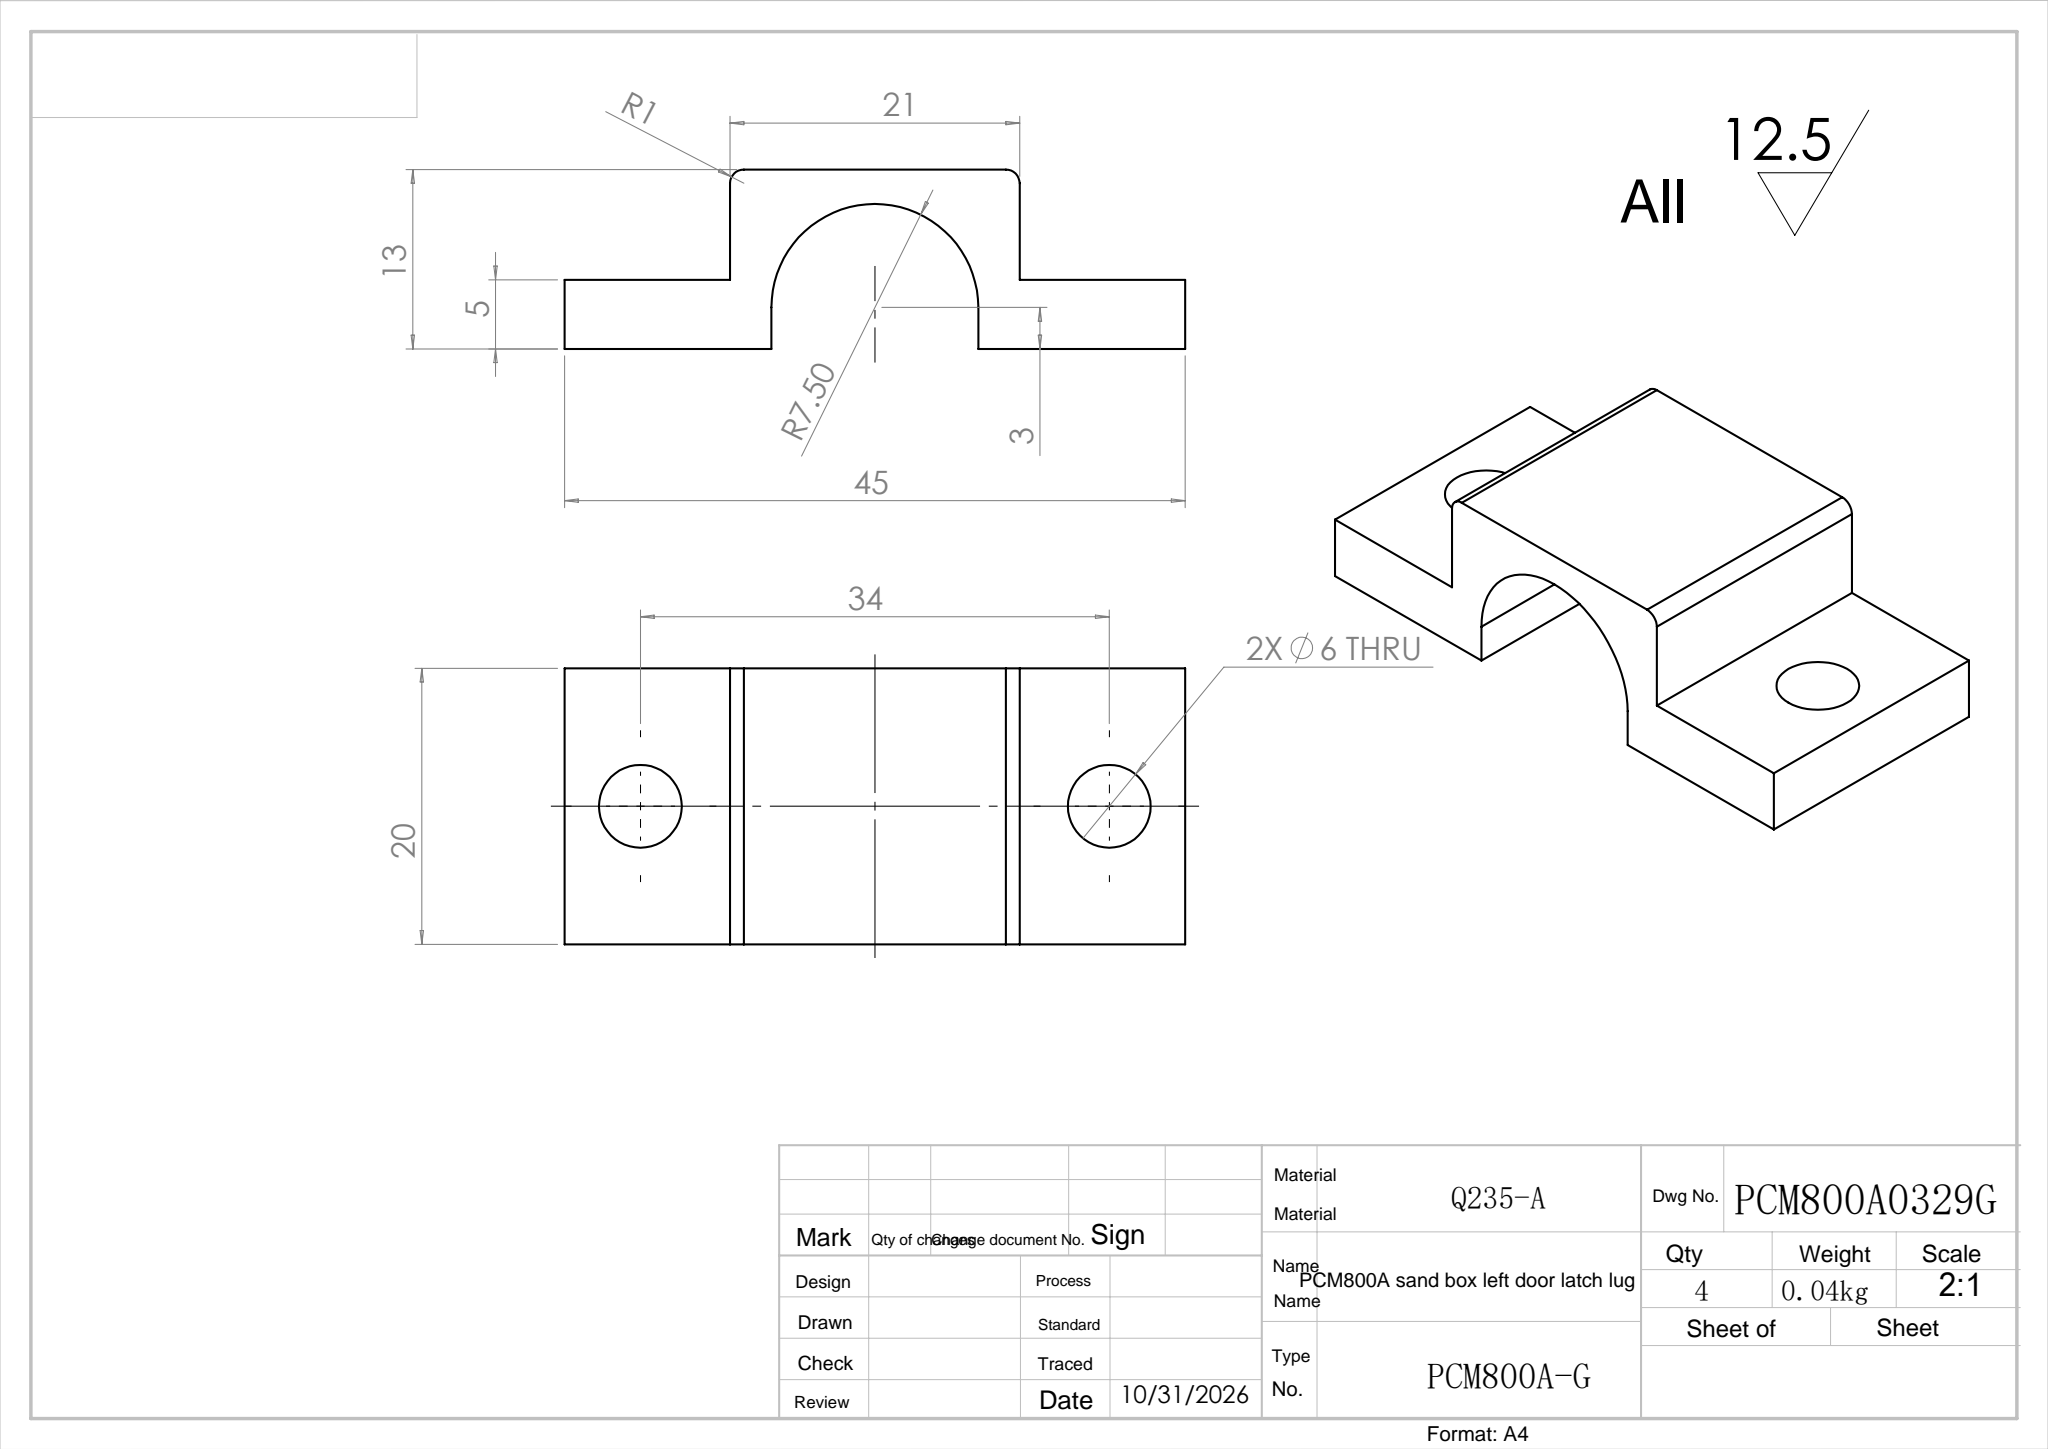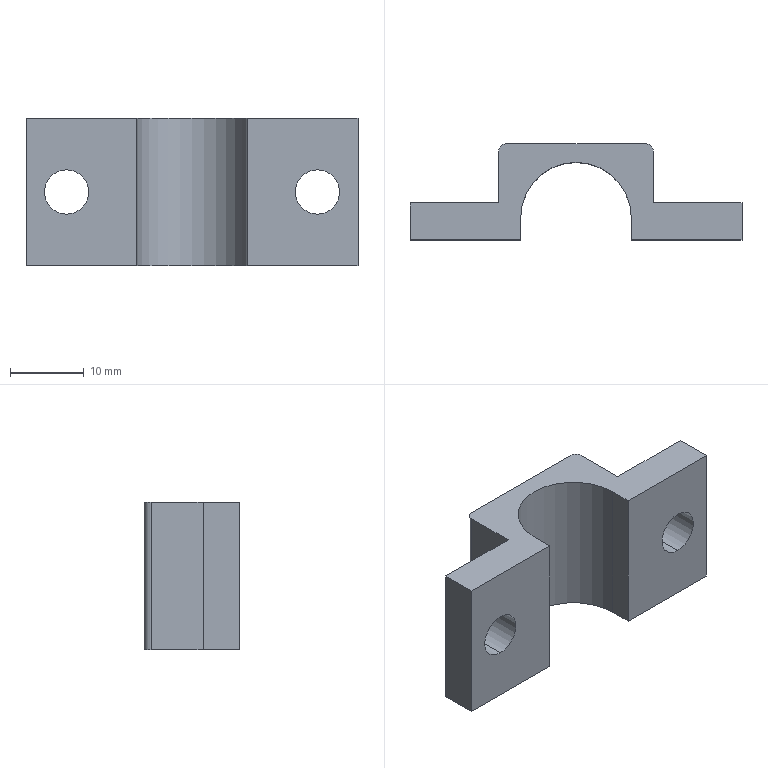Part | SolidWorks | features Extrusion 1, Fillet 1, ICE 1 | 1 solid | 20 faces | box 45 x 13 x 20 mm | volume 4902 mm3 | plane 13 | cylinder 7 | commonest cylinder face diameters 6 x4 2 x2 15 x1
STEP:
#1=CARTESIAN_POINT('',(39.5,-5.,7.));
#2=VERTEX_POINT('',#1);
#3=CARTESIAN_POINT('',(39.5,-5.,13.));
#4=VERTEX_POINT('',#3);
#5=CARTESIAN_POINT('',(39.5,-5.,10.));
#6=DIRECTION('',(0.,1.,0.));
#7=DIRECTION('',(0.,0.,1.));
#8=AXIS2_PLACEMENT_3D('',#5,#6,#7);
#9=CIRCLE('',#8,3.);
#10=EDGE_CURVE('',#2,#4,#9,.T.);
#11=ORIENTED_EDGE('',*,*,#10,.F.);
#12=CARTESIAN_POINT('',(39.5,0.,7.));
#13=VERTEX_POINT('',#12);
#14=CARTESIAN_POINT('',(39.5,-5.,7.));
#15=DIRECTION('',(0.,1.,0.));
#16=VECTOR('',#15,1000.);
#17=LINE('',#14,#16);
#18=EDGE_CURVE('',#2,#13,#17,.T.);
#19=ORIENTED_EDGE('',*,*,#18,.T.);
#20=CARTESIAN_POINT('',(39.5,0.,13.));
#21=VERTEX_POINT('',#20);
#22=CARTESIAN_POINT('',(39.5,0.,10.));
#23=DIRECTION('',(0.,1.,0.));
#24=DIRECTION('',(0.,0.,1.));
#25=AXIS2_PLACEMENT_3D('',#22,#23,#24);
#26=CIRCLE('',#25,3.);
#27=EDGE_CURVE('',#13,#21,#26,.T.);
#28=ORIENTED_EDGE('',*,*,#27,.T.);
#29=CARTESIAN_POINT('',(39.5,-5.,13.));
#30=DIRECTION('',(0.,1.,0.));
#31=VECTOR('',#30,1000.);
#32=LINE('',#29,#31);
#33=EDGE_CURVE('',#4,#21,#32,.T.);
#34=ORIENTED_EDGE('',*,*,#33,.F.);
#35=EDGE_LOOP('',(#11,#19,#28,#34));
#36=FACE_OUTER_BOUND('',#35,.T.);
#37=CARTESIAN_POINT('',(39.5,-5.,10.));
#38=DIRECTION('',(0.,1.,0.));
#39=DIRECTION('',(0.,0.,1.));
#40=AXIS2_PLACEMENT_3D('',#37,#38,#39);
#41=CYLINDRICAL_SURFACE('',#40,3.);
#42=ADVANCED_FACE('',(#36),#41,.F.);
#43=CARTESIAN_POINT('',(5.5,-5.,7.));
#44=VERTEX_POINT('',#43);
#45=CARTESIAN_POINT('',(5.5,-5.,13.));
#46=VERTEX_POINT('',#45);
#47=CARTESIAN_POINT('',(5.5,-5.,10.));
#48=DIRECTION('',(0.,1.,0.));
#49=DIRECTION('',(0.,0.,1.));
#50=AXIS2_PLACEMENT_3D('',#47,#48,#49);
#51=CIRCLE('',#50,3.);
#52=EDGE_CURVE('',#44,#46,#51,.T.);
#53=ORIENTED_EDGE('',*,*,#52,.F.);
#54=CARTESIAN_POINT('',(5.5,0.,7.));
#55=VERTEX_POINT('',#54);
#56=CARTESIAN_POINT('',(5.5,-5.,7.));
#57=DIRECTION('',(0.,1.,0.));
#58=VECTOR('',#57,1000.);
#59=LINE('',#56,#58);
#60=EDGE_CURVE('',#44,#55,#59,.T.);
#61=ORIENTED_EDGE('',*,*,#60,.T.);
#62=CARTESIAN_POINT('',(5.5,0.,13.));
#63=VERTEX_POINT('',#62);
#64=CARTESIAN_POINT('',(5.5,0.,10.));
#65=DIRECTION('',(0.,1.,0.));
#66=DIRECTION('',(0.,0.,1.));
#67=AXIS2_PLACEMENT_3D('',#64,#65,#66);
#68=CIRCLE('',#67,3.);
#69=EDGE_CURVE('',#55,#63,#68,.T.);
#70=ORIENTED_EDGE('',*,*,#69,.T.);
#71=CARTESIAN_POINT('',(5.5,-5.,13.));
#72=DIRECTION('',(0.,1.,0.));
#73=VECTOR('',#72,1000.);
#74=LINE('',#71,#73);
#75=EDGE_CURVE('',#46,#63,#74,.T.);
#76=ORIENTED_EDGE('',*,*,#75,.F.);
#77=EDGE_LOOP('',(#53,#61,#70,#76));
#78=FACE_OUTER_BOUND('',#77,.T.);
#79=CARTESIAN_POINT('',(5.5,-5.,10.));
#80=DIRECTION('',(0.,1.,0.));
#81=DIRECTION('',(0.,0.,1.));
#82=AXIS2_PLACEMENT_3D('',#79,#80,#81);
#83=CYLINDRICAL_SURFACE('',#82,3.);
#84=ADVANCED_FACE('',(#78),#83,.F.);
#85=CARTESIAN_POINT('',(0.,0.,0.));
#86=VERTEX_POINT('',#85);
#87=CARTESIAN_POINT('',(0.,-5.,0.));
#88=VERTEX_POINT('',#87);
#89=CARTESIAN_POINT('',(0.,-5.,0.));
#90=DIRECTION('',(0.,-1.,0.));
#91=VECTOR('',#90,1000.);
#92=LINE('',#89,#91);
#93=EDGE_CURVE('',#86,#88,#92,.T.);
#94=ORIENTED_EDGE('',*,*,#93,.T.);
#95=CARTESIAN_POINT('',(0.,-5.,20.));
#96=VERTEX_POINT('',#95);
#97=CARTESIAN_POINT('',(0.,-5.,20.));
#98=DIRECTION('',(0.,0.,-1.));
#99=VECTOR('',#98,1000.);
#100=LINE('',#97,#99);
#101=EDGE_CURVE('',#96,#88,#100,.T.);
#102=ORIENTED_EDGE('',*,*,#101,.F.);
#103=CARTESIAN_POINT('',(0.,0.,20.));
#104=VERTEX_POINT('',#103);
#105=CARTESIAN_POINT('',(0.,-5.,20.));
#106=DIRECTION('',(0.,-1.,0.));
#107=VECTOR('',#106,1000.);
#108=LINE('',#105,#107);
#109=EDGE_CURVE('',#104,#96,#108,.T.);
#110=ORIENTED_EDGE('',*,*,#109,.F.);
#111=CARTESIAN_POINT('',(0.,0.,20.));
#112=DIRECTION('',(0.,0.,-1.));
#113=VECTOR('',#112,1000.);
#114=LINE('',#111,#113);
#115=EDGE_CURVE('',#104,#86,#114,.T.);
#116=ORIENTED_EDGE('',*,*,#115,.T.);
#117=EDGE_LOOP('',(#94,#102,#110,#116));
#118=FACE_OUTER_BOUND('',#117,.T.);
#119=CARTESIAN_POINT('',(0.,-5.,20.));
#120=DIRECTION('',(1.,0.,0.));
#121=DIRECTION('',(0.,0.,-1.));
#122=AXIS2_PLACEMENT_3D('',#119,#120,#121);
#123=PLANE('',#122);
#124=ADVANCED_FACE('',(#118),#123,.F.);
#125=CARTESIAN_POINT('',(5.5,-5.,10.));
#126=DIRECTION('',(0.,1.,0.));
#127=DIRECTION('',(0.,0.,1.));
#128=AXIS2_PLACEMENT_3D('',#125,#126,#127);
#129=CIRCLE('',#128,3.);
#130=EDGE_CURVE('',#46,#44,#129,.T.);
#131=ORIENTED_EDGE('',*,*,#130,.T.);
#132=ORIENTED_EDGE('',*,*,#52,.T.);
#133=EDGE_LOOP('',(#131,#132));
#134=FACE_BOUND('',#133,.T.);
#135=CARTESIAN_POINT('',(15.,-5.,0.));
#136=VERTEX_POINT('',#135);
#137=CARTESIAN_POINT('',(15.,-5.,0.));
#138=DIRECTION('',(1.,0.,0.));
#139=VECTOR('',#138,1000.);
#140=LINE('',#137,#139);
#141=EDGE_CURVE('',#88,#136,#140,.T.);
#142=ORIENTED_EDGE('',*,*,#141,.T.);
#143=CARTESIAN_POINT('',(15.,-5.,20.));
#144=VERTEX_POINT('',#143);
#145=CARTESIAN_POINT('',(15.,-5.,20.));
#146=DIRECTION('',(0.,0.,-1.));
#147=VECTOR('',#146,1000.);
#148=LINE('',#145,#147);
#149=EDGE_CURVE('',#144,#136,#148,.T.);
#150=ORIENTED_EDGE('',*,*,#149,.F.);
#151=CARTESIAN_POINT('',(15.,-5.,20.));
#152=DIRECTION('',(1.,0.,0.));
#153=VECTOR('',#152,1000.);
#154=LINE('',#151,#153);
#155=EDGE_CURVE('',#96,#144,#154,.T.);
#156=ORIENTED_EDGE('',*,*,#155,.F.);
#157=ORIENTED_EDGE('',*,*,#101,.T.);
#158=EDGE_LOOP('',(#142,#150,#156,#157));
#159=FACE_OUTER_BOUND('',#158,.T.);
#160=CARTESIAN_POINT('',(15.,-5.,20.));
#161=DIRECTION('',(0.,1.,0.));
#162=DIRECTION('',(-1.,0.,0.));
#163=AXIS2_PLACEMENT_3D('',#160,#161,#162);
#164=PLANE('',#163);
#165=ADVANCED_FACE('',(#134,#159),#164,.F.);
#166=CARTESIAN_POINT('',(15.,-2.,0.));
#167=VERTEX_POINT('',#166);
#168=CARTESIAN_POINT('',(15.,-2.,0.));
#169=DIRECTION('',(0.,1.,0.));
#170=VECTOR('',#169,1000.);
#171=LINE('',#168,#170);
#172=EDGE_CURVE('',#136,#167,#171,.T.);
#173=ORIENTED_EDGE('',*,*,#172,.T.);
#174=CARTESIAN_POINT('',(15.,-2.,20.));
#175=VERTEX_POINT('',#174);
#176=CARTESIAN_POINT('',(15.,-2.,20.));
#177=DIRECTION('',(0.,0.,-1.));
#178=VECTOR('',#177,1000.);
#179=LINE('',#176,#178);
#180=EDGE_CURVE('',#175,#167,#179,.T.);
#181=ORIENTED_EDGE('',*,*,#180,.F.);
#182=CARTESIAN_POINT('',(15.,-2.,20.));
#183=DIRECTION('',(0.,1.,0.));
#184=VECTOR('',#183,1000.);
#185=LINE('',#182,#184);
#186=EDGE_CURVE('',#144,#175,#185,.T.);
#187=ORIENTED_EDGE('',*,*,#186,.F.);
#188=ORIENTED_EDGE('',*,*,#149,.T.);
#189=EDGE_LOOP('',(#173,#181,#187,#188));
#190=FACE_OUTER_BOUND('',#189,.T.);
#191=CARTESIAN_POINT('',(15.,-2.,20.));
#192=DIRECTION('',(-1.,0.,0.));
#193=DIRECTION('',(0.,0.,1.));
#194=AXIS2_PLACEMENT_3D('',#191,#192,#193);
#195=PLANE('',#194);
#196=ADVANCED_FACE('',(#190),#195,.F.);
#197=CARTESIAN_POINT('',(30.,-2.,0.));
#198=VERTEX_POINT('',#197);
#199=CARTESIAN_POINT('',(22.5,-2.,0.));
#200=DIRECTION('',(0.,0.,-1.));
#201=DIRECTION('',(1.,0.,0.));
#202=AXIS2_PLACEMENT_3D('',#199,#200,#201);
#203=CIRCLE('',#202,7.5);
#204=EDGE_CURVE('',#167,#198,#203,.T.);
#205=ORIENTED_EDGE('',*,*,#204,.T.);
#206=CARTESIAN_POINT('',(30.,-2.,20.));
#207=VERTEX_POINT('',#206);
#208=CARTESIAN_POINT('',(30.,-2.,20.));
#209=DIRECTION('',(0.,0.,-1.));
#210=VECTOR('',#209,1000.);
#211=LINE('',#208,#210);
#212=EDGE_CURVE('',#207,#198,#211,.T.);
#213=ORIENTED_EDGE('',*,*,#212,.F.);
#214=CARTESIAN_POINT('',(22.5,-2.,20.));
#215=DIRECTION('',(0.,0.,-1.));
#216=DIRECTION('',(1.,0.,0.));
#217=AXIS2_PLACEMENT_3D('',#214,#215,#216);
#218=CIRCLE('',#217,7.5);
#219=EDGE_CURVE('',#175,#207,#218,.T.);
#220=ORIENTED_EDGE('',*,*,#219,.F.);
#221=ORIENTED_EDGE('',*,*,#180,.T.);
#222=EDGE_LOOP('',(#205,#213,#220,#221));
#223=FACE_OUTER_BOUND('',#222,.T.);
#224=CARTESIAN_POINT('',(22.5,-2.,20.));
#225=DIRECTION('',(0.,0.,-1.));
#226=DIRECTION('',(-1.,0.,0.));
#227=AXIS2_PLACEMENT_3D('',#224,#225,#226);
#228=CYLINDRICAL_SURFACE('',#227,7.5);
#229=ADVANCED_FACE('',(#223),#228,.F.);
#230=CARTESIAN_POINT('',(30.,-5.,0.));
#231=VERTEX_POINT('',#230);
#232=CARTESIAN_POINT('',(30.,-2.,0.));
#233=DIRECTION('',(0.,-1.,0.));
#234=VECTOR('',#233,1000.);
#235=LINE('',#232,#234);
#236=EDGE_CURVE('',#198,#231,#235,.T.);
#237=ORIENTED_EDGE('',*,*,#236,.T.);
#238=CARTESIAN_POINT('',(30.,-5.,20.));
#239=VERTEX_POINT('',#238);
#240=CARTESIAN_POINT('',(30.,-5.,20.));
#241=DIRECTION('',(0.,0.,-1.));
#242=VECTOR('',#241,1000.);
#243=LINE('',#240,#242);
#244=EDGE_CURVE('',#239,#231,#243,.T.);
#245=ORIENTED_EDGE('',*,*,#244,.F.);
#246=CARTESIAN_POINT('',(30.,-2.,20.));
#247=DIRECTION('',(0.,-1.,0.));
#248=VECTOR('',#247,1000.);
#249=LINE('',#246,#248);
#250=EDGE_CURVE('',#207,#239,#249,.T.);
#251=ORIENTED_EDGE('',*,*,#250,.F.);
#252=ORIENTED_EDGE('',*,*,#212,.T.);
#253=EDGE_LOOP('',(#237,#245,#251,#252));
#254=FACE_OUTER_BOUND('',#253,.T.);
#255=CARTESIAN_POINT('',(30.,-2.,20.));
#256=DIRECTION('',(1.,0.,0.));
#257=DIRECTION('',(0.,0.,-1.));
#258=AXIS2_PLACEMENT_3D('',#255,#256,#257);
#259=PLANE('',#258);
#260=ADVANCED_FACE('',(#254),#259,.F.);
#261=CARTESIAN_POINT('',(39.5,-5.,10.));
#262=DIRECTION('',(0.,1.,0.));
#263=DIRECTION('',(0.,0.,1.));
#264=AXIS2_PLACEMENT_3D('',#261,#262,#263);
#265=CIRCLE('',#264,3.);
#266=EDGE_CURVE('',#4,#2,#265,.T.);
#267=ORIENTED_EDGE('',*,*,#266,.T.);
#268=ORIENTED_EDGE('',*,*,#10,.T.);
#269=EDGE_LOOP('',(#267,#268));
#270=FACE_BOUND('',#269,.T.);
#271=CARTESIAN_POINT('',(45.,-5.,0.));
#272=VERTEX_POINT('',#271);
#273=CARTESIAN_POINT('',(45.,-5.,0.));
#274=DIRECTION('',(1.,0.,0.));
#275=VECTOR('',#274,1000.);
#276=LINE('',#273,#275);
#277=EDGE_CURVE('',#231,#272,#276,.T.);
#278=ORIENTED_EDGE('',*,*,#277,.T.);
#279=CARTESIAN_POINT('',(45.,-5.,20.));
#280=VERTEX_POINT('',#279);
#281=CARTESIAN_POINT('',(45.,-5.,20.));
#282=DIRECTION('',(0.,0.,-1.));
#283=VECTOR('',#282,1000.);
#284=LINE('',#281,#283);
#285=EDGE_CURVE('',#280,#272,#284,.T.);
#286=ORIENTED_EDGE('',*,*,#285,.F.);
#287=CARTESIAN_POINT('',(45.,-5.,20.));
#288=DIRECTION('',(1.,0.,0.));
#289=VECTOR('',#288,1000.);
#290=LINE('',#287,#289);
#291=EDGE_CURVE('',#239,#280,#290,.T.);
#292=ORIENTED_EDGE('',*,*,#291,.F.);
#293=ORIENTED_EDGE('',*,*,#244,.T.);
#294=EDGE_LOOP('',(#278,#286,#292,#293));
#295=FACE_OUTER_BOUND('',#294,.T.);
#296=CARTESIAN_POINT('',(45.,-5.,20.));
#297=DIRECTION('',(0.,1.,0.));
#298=DIRECTION('',(-1.,0.,0.));
#299=AXIS2_PLACEMENT_3D('',#296,#297,#298);
#300=PLANE('',#299);
#301=ADVANCED_FACE('',(#270,#295),#300,.F.);
#302=CARTESIAN_POINT('',(45.,0.,0.));
#303=VERTEX_POINT('',#302);
#304=CARTESIAN_POINT('',(45.,0.,0.));
#305=DIRECTION('',(0.,1.,0.));
#306=VECTOR('',#305,1000.);
#307=LINE('',#304,#306);
#308=EDGE_CURVE('',#272,#303,#307,.T.);
#309=ORIENTED_EDGE('',*,*,#308,.T.);
#310=CARTESIAN_POINT('',(45.,0.,20.));
#311=VERTEX_POINT('',#310);
#312=CARTESIAN_POINT('',(45.,0.,20.));
#313=DIRECTION('',(0.,0.,-1.));
#314=VECTOR('',#313,1000.);
#315=LINE('',#312,#314);
#316=EDGE_CURVE('',#311,#303,#315,.T.);
#317=ORIENTED_EDGE('',*,*,#316,.F.);
#318=CARTESIAN_POINT('',(45.,0.,20.));
#319=DIRECTION('',(0.,1.,0.));
#320=VECTOR('',#319,1000.);
#321=LINE('',#318,#320);
#322=EDGE_CURVE('',#280,#311,#321,.T.);
#323=ORIENTED_EDGE('',*,*,#322,.F.);
#324=ORIENTED_EDGE('',*,*,#285,.T.);
#325=EDGE_LOOP('',(#309,#317,#323,#324));
#326=FACE_OUTER_BOUND('',#325,.T.);
#327=CARTESIAN_POINT('',(45.,0.,20.));
#328=DIRECTION('',(-1.,0.,0.));
#329=DIRECTION('',(0.,0.,1.));
#330=AXIS2_PLACEMENT_3D('',#327,#328,#329);
#331=PLANE('',#330);
#332=ADVANCED_FACE('',(#326),#331,.F.);
#333=CARTESIAN_POINT('',(39.5,0.,10.));
#334=DIRECTION('',(0.,1.,0.));
#335=DIRECTION('',(0.,0.,1.));
#336=AXIS2_PLACEMENT_3D('',#333,#334,#335);
#337=CIRCLE('',#336,3.);
#338=EDGE_CURVE('',#21,#13,#337,.T.);
#339=ORIENTED_EDGE('',*,*,#338,.F.);
#340=ORIENTED_EDGE('',*,*,#27,.F.);
#341=EDGE_LOOP('',(#339,#340));
#342=FACE_BOUND('',#341,.T.);
#343=CARTESIAN_POINT('',(33.,0.,0.));
#344=VERTEX_POINT('',#343);
#345=CARTESIAN_POINT('',(33.,0.,0.));
#346=DIRECTION('',(-1.,0.,0.));
#347=VECTOR('',#346,1000.);
#348=LINE('',#345,#347);
#349=EDGE_CURVE('',#303,#344,#348,.T.);
#350=ORIENTED_EDGE('',*,*,#349,.T.);
#351=CARTESIAN_POINT('',(33.,0.,20.));
#352=VERTEX_POINT('',#351);
#353=CARTESIAN_POINT('',(33.,0.,20.));
#354=DIRECTION('',(0.,0.,-1.));
#355=VECTOR('',#354,1000.);
#356=LINE('',#353,#355);
#357=EDGE_CURVE('',#352,#344,#356,.T.);
#358=ORIENTED_EDGE('',*,*,#357,.F.);
#359=CARTESIAN_POINT('',(33.,0.,20.));
#360=DIRECTION('',(-1.,0.,0.));
#361=VECTOR('',#360,1000.);
#362=LINE('',#359,#361);
#363=EDGE_CURVE('',#311,#352,#362,.T.);
#364=ORIENTED_EDGE('',*,*,#363,.F.);
#365=ORIENTED_EDGE('',*,*,#316,.T.);
#366=EDGE_LOOP('',(#350,#358,#364,#365));
#367=FACE_OUTER_BOUND('',#366,.T.);
#368=CARTESIAN_POINT('',(33.,0.,20.));
#369=DIRECTION('',(0.,-1.,0.));
#370=DIRECTION('',(0.,0.,-1.));
#371=AXIS2_PLACEMENT_3D('',#368,#369,#370);
#372=PLANE('',#371);
#373=ADVANCED_FACE('',(#342,#367),#372,.F.);
#374=CARTESIAN_POINT('',(33.,7.,0.));
#375=VERTEX_POINT('',#374);
#376=CARTESIAN_POINT('',(33.,8.,0.));
#377=DIRECTION('',(0.,1.,0.));
#378=VECTOR('',#377,1000.);
#379=LINE('',#376,#378);
#380=EDGE_CURVE('',#344,#375,#379,.T.);
#381=ORIENTED_EDGE('',*,*,#380,.T.);
#382=CARTESIAN_POINT('',(33.,7.,20.));
#383=VERTEX_POINT('',#382);
#384=CARTESIAN_POINT('',(33.,7.,20.));
#385=DIRECTION('',(0.,0.,1.));
#386=VECTOR('',#385,1000.);
#387=LINE('',#384,#386);
#388=EDGE_CURVE('',#375,#383,#387,.T.);
#389=ORIENTED_EDGE('',*,*,#388,.T.);
#390=CARTESIAN_POINT('',(33.,8.,20.));
#391=DIRECTION('',(0.,1.,0.));
#392=VECTOR('',#391,1000.);
#393=LINE('',#390,#392);
#394=EDGE_CURVE('',#352,#383,#393,.T.);
#395=ORIENTED_EDGE('',*,*,#394,.F.);
#396=ORIENTED_EDGE('',*,*,#357,.T.);
#397=EDGE_LOOP('',(#381,#389,#395,#396));
#398=FACE_OUTER_BOUND('',#397,.T.);
#399=CARTESIAN_POINT('',(33.,8.,20.));
#400=DIRECTION('',(-1.,0.,0.));
#401=DIRECTION('',(0.,-1.,0.));
#402=AXIS2_PLACEMENT_3D('',#399,#400,#401);
#403=PLANE('',#402);
#404=ADVANCED_FACE('',(#398),#403,.F.);
#405=CARTESIAN_POINT('',(32.,8.,20.));
#406=VERTEX_POINT('',#405);
#407=CARTESIAN_POINT('',(13.,8.,20.));
#408=VERTEX_POINT('',#407);
#409=CARTESIAN_POINT('',(12.,8.,20.));
#410=DIRECTION('',(-1.,0.,0.));
#411=VECTOR('',#410,1000.);
#412=LINE('',#409,#411);
#413=EDGE_CURVE('',#406,#408,#412,.T.);
#414=ORIENTED_EDGE('',*,*,#413,.F.);
#415=CARTESIAN_POINT('',(32.,8.,0.));
#416=VERTEX_POINT('',#415);
#417=CARTESIAN_POINT('',(32.,8.,20.));
#418=DIRECTION('',(0.,0.,-1.));
#419=VECTOR('',#418,1000.);
#420=LINE('',#417,#419);
#421=EDGE_CURVE('',#406,#416,#420,.T.);
#422=ORIENTED_EDGE('',*,*,#421,.T.);
#423=CARTESIAN_POINT('',(13.,8.,0.));
#424=VERTEX_POINT('',#423);
#425=CARTESIAN_POINT('',(12.,8.,0.));
#426=DIRECTION('',(-1.,0.,0.));
#427=VECTOR('',#426,1000.);
#428=LINE('',#425,#427);
#429=EDGE_CURVE('',#416,#424,#428,.T.);
#430=ORIENTED_EDGE('',*,*,#429,.T.);
#431=CARTESIAN_POINT('',(13.,8.,20.));
#432=DIRECTION('',(0.,0.,1.));
#433=VECTOR('',#432,1000.);
#434=LINE('',#431,#433);
#435=EDGE_CURVE('',#424,#408,#434,.T.);
#436=ORIENTED_EDGE('',*,*,#435,.T.);
#437=EDGE_LOOP('',(#414,#422,#430,#436));
#438=FACE_OUTER_BOUND('',#437,.T.);
#439=CARTESIAN_POINT('',(12.,8.,20.));
#440=DIRECTION('',(0.,-1.,0.));
#441=DIRECTION('',(0.,0.,-1.));
#442=AXIS2_PLACEMENT_3D('',#439,#440,#441);
#443=PLANE('',#442);
#444=ADVANCED_FACE('',(#438),#443,.F.);
#445=CARTESIAN_POINT('',(12.,7.,20.));
#446=VERTEX_POINT('',#445);
#447=CARTESIAN_POINT('',(12.,0.,20.));
#448=VERTEX_POINT('',#447);
#449=CARTESIAN_POINT('',(12.,0.,20.));
#450=DIRECTION('',(0.,-1.,0.));
#451=VECTOR('',#450,1000.);
#452=LINE('',#449,#451);
#453=EDGE_CURVE('',#446,#448,#452,.T.);
#454=ORIENTED_EDGE('',*,*,#453,.F.);
#455=CARTESIAN_POINT('',(12.,7.,0.));
#456=VERTEX_POINT('',#455);
#457=CARTESIAN_POINT('',(12.,7.,20.));
#458=DIRECTION('',(0.,0.,-1.));
#459=VECTOR('',#458,1000.);
#460=LINE('',#457,#459);
#461=EDGE_CURVE('',#446,#456,#460,.T.);
#462=ORIENTED_EDGE('',*,*,#461,.T.);
#463=CARTESIAN_POINT('',(12.,0.,0.));
#464=VERTEX_POINT('',#463);
#465=CARTESIAN_POINT('',(12.,0.,0.));
#466=DIRECTION('',(0.,-1.,0.));
#467=VECTOR('',#466,1000.);
#468=LINE('',#465,#467);
#469=EDGE_CURVE('',#456,#464,#468,.T.);
#470=ORIENTED_EDGE('',*,*,#469,.T.);
#471=CARTESIAN_POINT('',(12.,0.,20.));
#472=DIRECTION('',(0.,0.,-1.));
#473=VECTOR('',#472,1000.);
#474=LINE('',#471,#473);
#475=EDGE_CURVE('',#448,#464,#474,.T.);
#476=ORIENTED_EDGE('',*,*,#475,.F.);
#477=EDGE_LOOP('',(#454,#462,#470,#476));
#478=FACE_OUTER_BOUND('',#477,.T.);
#479=CARTESIAN_POINT('',(12.,0.,20.));
#480=DIRECTION('',(1.,0.,0.));
#481=DIRECTION('',(0.,1.,0.));
#482=AXIS2_PLACEMENT_3D('',#479,#480,#481);
#483=PLANE('',#482);
#484=ADVANCED_FACE('',(#478),#483,.F.);
#485=CARTESIAN_POINT('',(5.5,0.,10.));
#486=DIRECTION('',(0.,1.,0.));
#487=DIRECTION('',(0.,0.,1.));
#488=AXIS2_PLACEMENT_3D('',#485,#486,#487);
#489=CIRCLE('',#488,3.);
#490=EDGE_CURVE('',#63,#55,#489,.T.);
#491=ORIENTED_EDGE('',*,*,#490,.F.);
#492=ORIENTED_EDGE('',*,*,#69,.F.);
#493=EDGE_LOOP('',(#491,#492));
#494=FACE_BOUND('',#493,.T.);
#495=CARTESIAN_POINT('',(0.,0.,0.));
#496=DIRECTION('',(-1.,0.,0.));
#497=VECTOR('',#496,1000.);
#498=LINE('',#495,#497);
#499=EDGE_CURVE('',#464,#86,#498,.T.);
#500=ORIENTED_EDGE('',*,*,#499,.T.);
#501=ORIENTED_EDGE('',*,*,#115,.F.);
#502=CARTESIAN_POINT('',(0.,0.,20.));
#503=DIRECTION('',(-1.,0.,0.));
#504=VECTOR('',#503,1000.);
#505=LINE('',#502,#504);
#506=EDGE_CURVE('',#448,#104,#505,.T.);
#507=ORIENTED_EDGE('',*,*,#506,.F.);
#508=ORIENTED_EDGE('',*,*,#475,.T.);
#509=EDGE_LOOP('',(#500,#501,#507,#508));
#510=FACE_OUTER_BOUND('',#509,.T.);
#511=CARTESIAN_POINT('',(0.,0.,20.));
#512=DIRECTION('',(0.,-1.,0.));
#513=DIRECTION('',(0.,0.,-1.));
#514=AXIS2_PLACEMENT_3D('',#511,#512,#513);
#515=PLANE('',#514);
#516=ADVANCED_FACE('',(#494,#510),#515,.F.);
#517=ORIENTED_EDGE('',*,*,#394,.T.);
#518=CARTESIAN_POINT('',(32.,7.,20.));
#519=DIRECTION('',(0.,0.,1.));
#520=DIRECTION('',(1.,0.,0.));
#521=AXIS2_PLACEMENT_3D('',#518,#519,#520);
#522=CIRCLE('',#521,1.);
#523=EDGE_CURVE('',#383,#406,#522,.T.);
#524=ORIENTED_EDGE('',*,*,#523,.T.);
#525=ORIENTED_EDGE('',*,*,#413,.T.);
#526=CARTESIAN_POINT('',(13.,7.,20.));
#527=DIRECTION('',(0.,0.,1.));
#528=DIRECTION('',(1.,0.,0.));
#529=AXIS2_PLACEMENT_3D('',#526,#527,#528);
#530=CIRCLE('',#529,1.);
#531=EDGE_CURVE('',#408,#446,#530,.T.);
#532=ORIENTED_EDGE('',*,*,#531,.T.);
#533=ORIENTED_EDGE('',*,*,#453,.T.);
#534=ORIENTED_EDGE('',*,*,#506,.T.);
#535=ORIENTED_EDGE('',*,*,#109,.T.);
#536=ORIENTED_EDGE('',*,*,#155,.T.);
#537=ORIENTED_EDGE('',*,*,#186,.T.);
#538=ORIENTED_EDGE('',*,*,#219,.T.);
#539=ORIENTED_EDGE('',*,*,#250,.T.);
#540=ORIENTED_EDGE('',*,*,#291,.T.);
#541=ORIENTED_EDGE('',*,*,#322,.T.);
#542=ORIENTED_EDGE('',*,*,#363,.T.);
#543=EDGE_LOOP('',(#517,#524,#525,#532,#533,#534,#535,#536,#537,#538,#539,#540,#541,#542));
#544=FACE_OUTER_BOUND('',#543,.T.);
#545=CARTESIAN_POINT('',(22.5,-2.,20.));
#546=DIRECTION('',(0.,0.,1.));
#547=DIRECTION('',(1.,0.,0.));
#548=AXIS2_PLACEMENT_3D('',#545,#546,#547);
#549=PLANE('',#548);
#550=ADVANCED_FACE('',(#544),#549,.T.);
#551=ORIENTED_EDGE('',*,*,#429,.F.);
#552=CARTESIAN_POINT('',(32.,7.,0.));
#553=DIRECTION('',(0.,0.,-1.));
#554=DIRECTION('',(1.,0.,0.));
#555=AXIS2_PLACEMENT_3D('',#552,#553,#554);
#556=CIRCLE('',#555,1.);
#557=EDGE_CURVE('',#416,#375,#556,.T.);
#558=ORIENTED_EDGE('',*,*,#557,.T.);
#559=ORIENTED_EDGE('',*,*,#380,.F.);
#560=ORIENTED_EDGE('',*,*,#349,.F.);
#561=ORIENTED_EDGE('',*,*,#308,.F.);
#562=ORIENTED_EDGE('',*,*,#277,.F.);
#563=ORIENTED_EDGE('',*,*,#236,.F.);
#564=ORIENTED_EDGE('',*,*,#204,.F.);
#565=ORIENTED_EDGE('',*,*,#172,.F.);
#566=ORIENTED_EDGE('',*,*,#141,.F.);
#567=ORIENTED_EDGE('',*,*,#93,.F.);
#568=ORIENTED_EDGE('',*,*,#499,.F.);
#569=ORIENTED_EDGE('',*,*,#469,.F.);
#570=CARTESIAN_POINT('',(13.,7.,0.));
#571=DIRECTION('',(0.,0.,-1.));
#572=DIRECTION('',(1.,0.,0.));
#573=AXIS2_PLACEMENT_3D('',#570,#571,#572);
#574=CIRCLE('',#573,1.);
#575=EDGE_CURVE('',#456,#424,#574,.T.);
#576=ORIENTED_EDGE('',*,*,#575,.T.);
#577=EDGE_LOOP('',(#551,#558,#559,#560,#561,#562,#563,#564,#565,#566,#567,#568,#569,#576));
#578=FACE_OUTER_BOUND('',#577,.T.);
#579=CARTESIAN_POINT('',(22.5,-2.,0.));
#580=DIRECTION('',(0.,0.,1.));
#581=DIRECTION('',(1.,0.,0.));
#582=AXIS2_PLACEMENT_3D('',#579,#580,#581);
#583=PLANE('',#582);
#584=ADVANCED_FACE('',(#578),#583,.F.);
#585=ORIENTED_EDGE('',*,*,#523,.F.);
#586=ORIENTED_EDGE('',*,*,#388,.F.);
#587=ORIENTED_EDGE('',*,*,#557,.F.);
#588=ORIENTED_EDGE('',*,*,#421,.F.);
#589=EDGE_LOOP('',(#585,#586,#587,#588));
#590=FACE_OUTER_BOUND('',#589,.T.);
#591=CARTESIAN_POINT('',(32.,7.,20.));
#592=DIRECTION('',(0.,0.,-1.));
#593=DIRECTION('',(-1.,0.,0.));
#594=AXIS2_PLACEMENT_3D('',#591,#592,#593);
#595=CYLINDRICAL_SURFACE('',#594,1.);
#596=ADVANCED_FACE('',(#590),#595,.T.);
#597=ORIENTED_EDGE('',*,*,#531,.F.);
#598=ORIENTED_EDGE('',*,*,#435,.F.);
#599=ORIENTED_EDGE('',*,*,#575,.F.);
#600=ORIENTED_EDGE('',*,*,#461,.F.);
#601=EDGE_LOOP('',(#597,#598,#599,#600));
#602=FACE_OUTER_BOUND('',#601,.T.);
#603=CARTESIAN_POINT('',(13.,7.,20.));
#604=DIRECTION('',(0.,0.,-1.));
#605=DIRECTION('',(-1.,0.,0.));
#606=AXIS2_PLACEMENT_3D('',#603,#604,#605);
#607=CYLINDRICAL_SURFACE('',#606,1.);
#608=ADVANCED_FACE('',(#602),#607,.T.);
#609=ORIENTED_EDGE('',*,*,#60,.F.);
#610=ORIENTED_EDGE('',*,*,#130,.F.);
#611=ORIENTED_EDGE('',*,*,#75,.T.);
#612=ORIENTED_EDGE('',*,*,#490,.T.);
#613=EDGE_LOOP('',(#609,#610,#611,#612));
#614=FACE_OUTER_BOUND('',#613,.T.);
#615=CARTESIAN_POINT('',(5.5,-5.,10.));
#616=DIRECTION('',(0.,1.,0.));
#617=DIRECTION('',(0.,0.,1.));
#618=AXIS2_PLACEMENT_3D('',#615,#616,#617);
#619=CYLINDRICAL_SURFACE('',#618,3.);
#620=ADVANCED_FACE('',(#614),#619,.F.);
#621=ORIENTED_EDGE('',*,*,#18,.F.);
#622=ORIENTED_EDGE('',*,*,#266,.F.);
#623=ORIENTED_EDGE('',*,*,#33,.T.);
#624=ORIENTED_EDGE('',*,*,#338,.T.);
#625=EDGE_LOOP('',(#621,#622,#623,#624));
#626=FACE_OUTER_BOUND('',#625,.T.);
#627=CARTESIAN_POINT('',(39.5,-5.,10.));
#628=DIRECTION('',(0.,1.,0.));
#629=DIRECTION('',(0.,0.,1.));
#630=AXIS2_PLACEMENT_3D('',#627,#628,#629);
#631=CYLINDRICAL_SURFACE('',#630,3.);
#632=ADVANCED_FACE('',(#626),#631,.F.);
#633=CLOSED_SHELL('',(#42,#84,#124,#165,#196,#229,#260,#301,#332,#373,#404,#444,#484,#516,#550,#584,#596,#608,#620,#632));
#634=MANIFOLD_SOLID_BREP('',#633);
#635=CARTESIAN_POINT('',(0.,0.,0.));
#636=DIRECTION('',(0.,0.,1.));
#637=DIRECTION('',(1.,0.,0.));
#638=AXIS2_PLACEMENT_3D('',#635,#636,#637);
#639=(LENGTH_UNIT()NAMED_UNIT(*)SI_UNIT(.MILLI.,.METRE.));
#640=UNCERTAINTY_MEASURE_WITH_UNIT(LENGTH_MEASURE(0.00001),#639,'','');
#641=(NAMED_UNIT(*)PLANE_ANGLE_UNIT()SI_UNIT($,.RADIAN.));
#642=(NAMED_UNIT(*)SI_UNIT($,.STERADIAN.)SOLID_ANGLE_UNIT());
#643=(GEOMETRIC_REPRESENTATION_CONTEXT(3)GLOBAL_UNCERTAINTY_ASSIGNED_CONTEXT((#640))GLOBAL_UNIT_ASSIGNED_CONTEXT((#639,#641,#642))REPRESENTATION_CONTEXT('',''));
#644=ADVANCED_BREP_SHAPE_REPRESENTATION('',(#634,#638),#643);